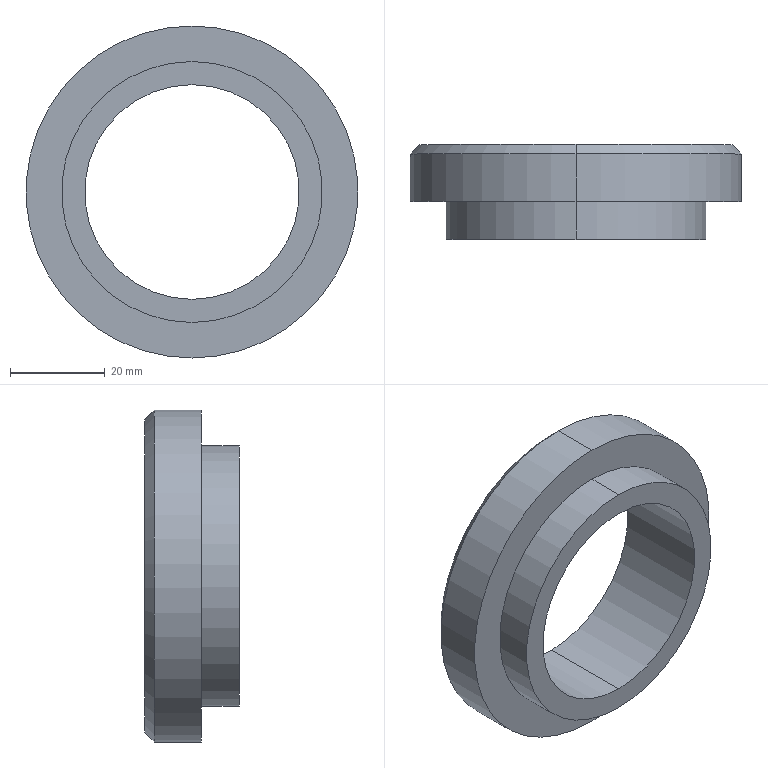Part | SolidWorks | features Chamfer 1, HoleWzd 1, Revolution 1 | 1 solid | 11 faces | box 70 x 20 x 70 mm | volume 32594 mm3 | cylinder 6 | plane 3 | cone 2 | commonest cylinder face diameters 45.25 x2 55 x2 70 x2
STEP:
#1=CARTESIAN_POINT('',(0.,0.,33.));
#2=VERTEX_POINT('',#1);
#3=CARTESIAN_POINT('',(0.,0.,-33.));
#4=VERTEX_POINT('',#3);
#5=CARTESIAN_POINT('',(0.,0.,0.));
#6=DIRECTION('',(0.,1.,0.));
#7=DIRECTION('',(0.,0.,1.));
#8=AXIS2_PLACEMENT_3D('',#5,#6,#7);
#9=CIRCLE('',#8,33.);
#10=EDGE_CURVE('',#2,#4,#9,.T.);
#11=ORIENTED_EDGE('',*,*,#10,.F.);
#12=CARTESIAN_POINT('',(0.,-2.,35.));
#13=VERTEX_POINT('',#12);
#14=CARTESIAN_POINT('',(0.,-2.,35.));
#15=DIRECTION('',(0.,-0.7071,0.7071));
#16=VECTOR('',#15,1000.);
#17=LINE('',#14,#16);
#18=EDGE_CURVE('',#2,#13,#17,.T.);
#19=ORIENTED_EDGE('',*,*,#18,.T.);
#20=CARTESIAN_POINT('',(0.,-2.,-35.));
#21=VERTEX_POINT('',#20);
#22=CARTESIAN_POINT('',(0.,-2.,0.));
#23=DIRECTION('',(0.,-1.,0.));
#24=DIRECTION('',(0.,0.,1.));
#25=AXIS2_PLACEMENT_3D('',#22,#23,#24);
#26=CIRCLE('',#25,35.);
#27=EDGE_CURVE('',#21,#13,#26,.T.);
#28=ORIENTED_EDGE('',*,*,#27,.F.);
#29=CARTESIAN_POINT('',(0.,-2.,-35.));
#30=DIRECTION('',(0.,-0.7071,-0.7071));
#31=VECTOR('',#30,1000.);
#32=LINE('',#29,#31);
#33=EDGE_CURVE('',#4,#21,#32,.T.);
#34=ORIENTED_EDGE('',*,*,#33,.F.);
#35=EDGE_LOOP('',(#11,#19,#28,#34));
#36=FACE_OUTER_BOUND('',#35,.T.);
#37=CARTESIAN_POINT('',(0.,-2.,0.));
#38=DIRECTION('',(0.,-1.,0.));
#39=DIRECTION('',(0.,0.,-1.));
#40=AXIS2_PLACEMENT_3D('',#37,#38,#39);
#41=CONICAL_SURFACE('',#40,35.,0.7854);
#42=ADVANCED_FACE('',(#36),#41,.T.);
#43=CARTESIAN_POINT('',(0.,-20.,22.625));
#44=VERTEX_POINT('',#43);
#45=CARTESIAN_POINT('',(0.,-20.,-22.625));
#46=VERTEX_POINT('',#45);
#47=CARTESIAN_POINT('',(0.,-20.,0.));
#48=DIRECTION('',(0.,-1.,0.));
#49=DIRECTION('',(0.,0.,-1.));
#50=AXIS2_PLACEMENT_3D('',#47,#48,#49);
#51=CIRCLE('',#50,22.625);
#52=EDGE_CURVE('',#44,#46,#51,.T.);
#53=ORIENTED_EDGE('',*,*,#52,.T.);
#54=CARTESIAN_POINT('',(0.,0.,-22.625));
#55=VERTEX_POINT('',#54);
#56=CARTESIAN_POINT('',(0.,0.,-22.625));
#57=DIRECTION('',(0.,1.,0.));
#58=VECTOR('',#57,1000.);
#59=LINE('',#56,#58);
#60=EDGE_CURVE('',#46,#55,#59,.T.);
#61=ORIENTED_EDGE('',*,*,#60,.T.);
#62=CARTESIAN_POINT('',(0.,0.,22.625));
#63=VERTEX_POINT('',#62);
#64=CARTESIAN_POINT('',(0.,0.,0.));
#65=DIRECTION('',(0.,1.,0.));
#66=DIRECTION('',(0.,0.,1.));
#67=AXIS2_PLACEMENT_3D('',#64,#65,#66);
#68=CIRCLE('',#67,22.625);
#69=EDGE_CURVE('',#55,#63,#68,.T.);
#70=ORIENTED_EDGE('',*,*,#69,.T.);
#71=CARTESIAN_POINT('',(0.,0.,22.625));
#72=DIRECTION('',(0.,1.,0.));
#73=VECTOR('',#72,1000.);
#74=LINE('',#71,#73);
#75=EDGE_CURVE('',#44,#63,#74,.T.);
#76=ORIENTED_EDGE('',*,*,#75,.F.);
#77=EDGE_LOOP('',(#53,#61,#70,#76));
#78=FACE_OUTER_BOUND('',#77,.T.);
#79=CARTESIAN_POINT('',(0.,0.,0.));
#80=DIRECTION('',(0.,1.,0.));
#81=DIRECTION('',(0.,0.,1.));
#82=AXIS2_PLACEMENT_3D('',#79,#80,#81);
#83=CYLINDRICAL_SURFACE('',#82,22.625);
#84=ADVANCED_FACE('',(#78),#83,.F.);
#85=CARTESIAN_POINT('',(0.,-12.,-27.5));
#86=VERTEX_POINT('',#85);
#87=CARTESIAN_POINT('',(0.,-12.,27.5));
#88=VERTEX_POINT('',#87);
#89=CARTESIAN_POINT('',(0.,-12.,0.));
#90=DIRECTION('',(0.,-1.,0.));
#91=DIRECTION('',(0.,0.,-1.));
#92=AXIS2_PLACEMENT_3D('',#89,#90,#91);
#93=CIRCLE('',#92,27.5);
#94=EDGE_CURVE('',#86,#88,#93,.T.);
#95=ORIENTED_EDGE('',*,*,#94,.T.);
#96=CARTESIAN_POINT('',(0.,-20.,27.5));
#97=VERTEX_POINT('',#96);
#98=CARTESIAN_POINT('',(0.,-20.,27.5));
#99=DIRECTION('',(0.,-1.,0.));
#100=VECTOR('',#99,1000.);
#101=LINE('',#98,#100);
#102=EDGE_CURVE('',#88,#97,#101,.T.);
#103=ORIENTED_EDGE('',*,*,#102,.T.);
#104=CARTESIAN_POINT('',(0.,-20.,-27.5));
#105=VERTEX_POINT('',#104);
#106=CARTESIAN_POINT('',(0.,-20.,0.));
#107=DIRECTION('',(0.,-1.,0.));
#108=DIRECTION('',(0.,0.,-1.));
#109=AXIS2_PLACEMENT_3D('',#106,#107,#108);
#110=CIRCLE('',#109,27.5);
#111=EDGE_CURVE('',#105,#97,#110,.T.);
#112=ORIENTED_EDGE('',*,*,#111,.F.);
#113=CARTESIAN_POINT('',(0.,-20.,-27.5));
#114=DIRECTION('',(0.,-1.,0.));
#115=VECTOR('',#114,1000.);
#116=LINE('',#113,#115);
#117=EDGE_CURVE('',#86,#105,#116,.T.);
#118=ORIENTED_EDGE('',*,*,#117,.F.);
#119=EDGE_LOOP('',(#95,#103,#112,#118));
#120=FACE_OUTER_BOUND('',#119,.T.);
#121=CARTESIAN_POINT('',(0.,-20.,0.));
#122=DIRECTION('',(0.,-1.,0.));
#123=DIRECTION('',(0.,0.,-1.));
#124=AXIS2_PLACEMENT_3D('',#121,#122,#123);
#125=CYLINDRICAL_SURFACE('',#124,27.5);
#126=ADVANCED_FACE('',(#120),#125,.T.);
#127=ORIENTED_EDGE('',*,*,#27,.T.);
#128=CARTESIAN_POINT('',(0.,-12.,35.));
#129=VERTEX_POINT('',#128);
#130=CARTESIAN_POINT('',(0.,-20.,35.));
#131=DIRECTION('',(0.,-1.,0.));
#132=VECTOR('',#131,1000.);
#133=LINE('',#130,#132);
#134=EDGE_CURVE('',#13,#129,#133,.T.);
#135=ORIENTED_EDGE('',*,*,#134,.T.);
#136=CARTESIAN_POINT('',(0.,-12.,-35.));
#137=VERTEX_POINT('',#136);
#138=CARTESIAN_POINT('',(0.,-12.,0.));
#139=DIRECTION('',(0.,-1.,0.));
#140=DIRECTION('',(0.,0.,-1.));
#141=AXIS2_PLACEMENT_3D('',#138,#139,#140);
#142=CIRCLE('',#141,35.);
#143=EDGE_CURVE('',#137,#129,#142,.T.);
#144=ORIENTED_EDGE('',*,*,#143,.F.);
#145=CARTESIAN_POINT('',(0.,-20.,-35.));
#146=DIRECTION('',(0.,-1.,0.));
#147=VECTOR('',#146,1000.);
#148=LINE('',#145,#147);
#149=EDGE_CURVE('',#21,#137,#148,.T.);
#150=ORIENTED_EDGE('',*,*,#149,.F.);
#151=EDGE_LOOP('',(#127,#135,#144,#150));
#152=FACE_OUTER_BOUND('',#151,.T.);
#153=CARTESIAN_POINT('',(0.,-20.,0.));
#154=DIRECTION('',(0.,-1.,0.));
#155=DIRECTION('',(0.,0.,-1.));
#156=AXIS2_PLACEMENT_3D('',#153,#154,#155);
#157=CYLINDRICAL_SURFACE('',#156,35.);
#158=ADVANCED_FACE('',(#152),#157,.T.);
#159=CARTESIAN_POINT('',(0.,0.,0.));
#160=DIRECTION('',(0.,1.,0.));
#161=DIRECTION('',(0.,0.,1.));
#162=AXIS2_PLACEMENT_3D('',#159,#160,#161);
#163=CIRCLE('',#162,33.);
#164=EDGE_CURVE('',#4,#2,#163,.T.);
#165=ORIENTED_EDGE('',*,*,#164,.T.);
#166=ORIENTED_EDGE('',*,*,#10,.T.);
#167=EDGE_LOOP('',(#165,#166));
#168=FACE_OUTER_BOUND('',#167,.T.);
#169=CARTESIAN_POINT('',(0.,0.,0.));
#170=DIRECTION('',(0.,1.,0.));
#171=DIRECTION('',(0.,0.,1.));
#172=AXIS2_PLACEMENT_3D('',#169,#170,#171);
#173=CIRCLE('',#172,22.625);
#174=EDGE_CURVE('',#63,#55,#173,.T.);
#175=ORIENTED_EDGE('',*,*,#174,.F.);
#176=ORIENTED_EDGE('',*,*,#69,.F.);
#177=EDGE_LOOP('',(#175,#176));
#178=FACE_BOUND('',#177,.T.);
#179=CARTESIAN_POINT('',(0.,0.,0.));
#180=DIRECTION('',(0.,1.,0.));
#181=DIRECTION('',(0.,0.,1.));
#182=AXIS2_PLACEMENT_3D('',#179,#180,#181);
#183=PLANE('',#182);
#184=ADVANCED_FACE('',(#168,#178),#183,.T.);
#185=ORIENTED_EDGE('',*,*,#134,.F.);
#186=CARTESIAN_POINT('',(0.,-2.,0.));
#187=DIRECTION('',(0.,-1.,0.));
#188=DIRECTION('',(0.,0.,1.));
#189=AXIS2_PLACEMENT_3D('',#186,#187,#188);
#190=CIRCLE('',#189,35.);
#191=EDGE_CURVE('',#13,#21,#190,.T.);
#192=ORIENTED_EDGE('',*,*,#191,.T.);
#193=ORIENTED_EDGE('',*,*,#149,.T.);
#194=CARTESIAN_POINT('',(0.,-12.,0.));
#195=DIRECTION('',(0.,-1.,0.));
#196=DIRECTION('',(0.,0.,-1.));
#197=AXIS2_PLACEMENT_3D('',#194,#195,#196);
#198=CIRCLE('',#197,35.);
#199=EDGE_CURVE('',#129,#137,#198,.T.);
#200=ORIENTED_EDGE('',*,*,#199,.F.);
#201=EDGE_LOOP('',(#185,#192,#193,#200));
#202=FACE_OUTER_BOUND('',#201,.T.);
#203=CARTESIAN_POINT('',(0.,-20.,0.));
#204=DIRECTION('',(0.,-1.,0.));
#205=DIRECTION('',(0.,0.,-1.));
#206=AXIS2_PLACEMENT_3D('',#203,#204,#205);
#207=CYLINDRICAL_SURFACE('',#206,35.);
#208=ADVANCED_FACE('',(#202),#207,.T.);
#209=ORIENTED_EDGE('',*,*,#143,.T.);
#210=ORIENTED_EDGE('',*,*,#199,.T.);
#211=EDGE_LOOP('',(#209,#210));
#212=FACE_OUTER_BOUND('',#211,.T.);
#213=ORIENTED_EDGE('',*,*,#94,.F.);
#214=CARTESIAN_POINT('',(0.,-12.,0.));
#215=DIRECTION('',(0.,-1.,0.));
#216=DIRECTION('',(0.,0.,-1.));
#217=AXIS2_PLACEMENT_3D('',#214,#215,#216);
#218=CIRCLE('',#217,27.5);
#219=EDGE_CURVE('',#88,#86,#218,.T.);
#220=ORIENTED_EDGE('',*,*,#219,.F.);
#221=EDGE_LOOP('',(#213,#220));
#222=FACE_BOUND('',#221,.T.);
#223=CARTESIAN_POINT('',(35.,-12.,0.));
#224=DIRECTION('',(0.,-1.,0.));
#225=DIRECTION('',(0.,0.,-1.));
#226=AXIS2_PLACEMENT_3D('',#223,#224,#225);
#227=PLANE('',#226);
#228=ADVANCED_FACE('',(#212,#222),#227,.T.);
#229=ORIENTED_EDGE('',*,*,#102,.F.);
#230=ORIENTED_EDGE('',*,*,#219,.T.);
#231=ORIENTED_EDGE('',*,*,#117,.T.);
#232=CARTESIAN_POINT('',(0.,-20.,0.));
#233=DIRECTION('',(0.,-1.,0.));
#234=DIRECTION('',(0.,0.,-1.));
#235=AXIS2_PLACEMENT_3D('',#232,#233,#234);
#236=CIRCLE('',#235,27.5);
#237=EDGE_CURVE('',#97,#105,#236,.T.);
#238=ORIENTED_EDGE('',*,*,#237,.F.);
#239=EDGE_LOOP('',(#229,#230,#231,#238));
#240=FACE_OUTER_BOUND('',#239,.T.);
#241=CARTESIAN_POINT('',(0.,-20.,0.));
#242=DIRECTION('',(0.,-1.,0.));
#243=DIRECTION('',(0.,0.,-1.));
#244=AXIS2_PLACEMENT_3D('',#241,#242,#243);
#245=CYLINDRICAL_SURFACE('',#244,27.5);
#246=ADVANCED_FACE('',(#240),#245,.T.);
#247=ORIENTED_EDGE('',*,*,#52,.F.);
#248=CARTESIAN_POINT('',(0.,-20.,0.));
#249=DIRECTION('',(0.,-1.,0.));
#250=DIRECTION('',(0.,0.,-1.));
#251=AXIS2_PLACEMENT_3D('',#248,#249,#250);
#252=CIRCLE('',#251,22.625);
#253=EDGE_CURVE('',#46,#44,#252,.T.);
#254=ORIENTED_EDGE('',*,*,#253,.F.);
#255=EDGE_LOOP('',(#247,#254));
#256=FACE_BOUND('',#255,.T.);
#257=ORIENTED_EDGE('',*,*,#111,.T.);
#258=ORIENTED_EDGE('',*,*,#237,.T.);
#259=EDGE_LOOP('',(#257,#258));
#260=FACE_OUTER_BOUND('',#259,.T.);
#261=CARTESIAN_POINT('',(27.5,-20.,0.));
#262=DIRECTION('',(0.,-1.,0.));
#263=DIRECTION('',(0.,0.,-1.));
#264=AXIS2_PLACEMENT_3D('',#261,#262,#263);
#265=PLANE('',#264);
#266=ADVANCED_FACE('',(#256,#260),#265,.T.);
#267=ORIENTED_EDGE('',*,*,#60,.F.);
#268=ORIENTED_EDGE('',*,*,#253,.T.);
#269=ORIENTED_EDGE('',*,*,#75,.T.);
#270=ORIENTED_EDGE('',*,*,#174,.T.);
#271=EDGE_LOOP('',(#267,#268,#269,#270));
#272=FACE_OUTER_BOUND('',#271,.T.);
#273=CARTESIAN_POINT('',(0.,0.,0.));
#274=DIRECTION('',(0.,1.,0.));
#275=DIRECTION('',(0.,0.,1.));
#276=AXIS2_PLACEMENT_3D('',#273,#274,#275);
#277=CYLINDRICAL_SURFACE('',#276,22.625);
#278=ADVANCED_FACE('',(#272),#277,.F.);
#279=ORIENTED_EDGE('',*,*,#18,.F.);
#280=ORIENTED_EDGE('',*,*,#164,.F.);
#281=ORIENTED_EDGE('',*,*,#33,.T.);
#282=ORIENTED_EDGE('',*,*,#191,.F.);
#283=EDGE_LOOP('',(#279,#280,#281,#282));
#284=FACE_OUTER_BOUND('',#283,.T.);
#285=CARTESIAN_POINT('',(0.,-2.,0.));
#286=DIRECTION('',(0.,-1.,0.));
#287=DIRECTION('',(0.,0.,-1.));
#288=AXIS2_PLACEMENT_3D('',#285,#286,#287);
#289=CONICAL_SURFACE('',#288,35.,0.7854);
#290=ADVANCED_FACE('',(#284),#289,.T.);
#291=CLOSED_SHELL('',(#42,#84,#126,#158,#184,#208,#228,#246,#266,#278,#290));
#292=MANIFOLD_SOLID_BREP('',#291);
#293=CARTESIAN_POINT('',(0.,0.,0.));
#294=DIRECTION('',(0.,0.,1.));
#295=DIRECTION('',(1.,0.,0.));
#296=AXIS2_PLACEMENT_3D('',#293,#294,#295);
#297=(LENGTH_UNIT()NAMED_UNIT(*)SI_UNIT(.MILLI.,.METRE.));
#298=UNCERTAINTY_MEASURE_WITH_UNIT(LENGTH_MEASURE(0.00001),#297,'','');
#299=(NAMED_UNIT(*)PLANE_ANGLE_UNIT()SI_UNIT($,.RADIAN.));
#300=(NAMED_UNIT(*)SI_UNIT($,.STERADIAN.)SOLID_ANGLE_UNIT());
#301=(GEOMETRIC_REPRESENTATION_CONTEXT(3)GLOBAL_UNCERTAINTY_ASSIGNED_CONTEXT((#298))GLOBAL_UNIT_ASSIGNED_CONTEXT((#297,#299,#300))REPRESENTATION_CONTEXT('',''));
#302=ADVANCED_BREP_SHAPE_REPRESENTATION('',(#292,#296),#301);